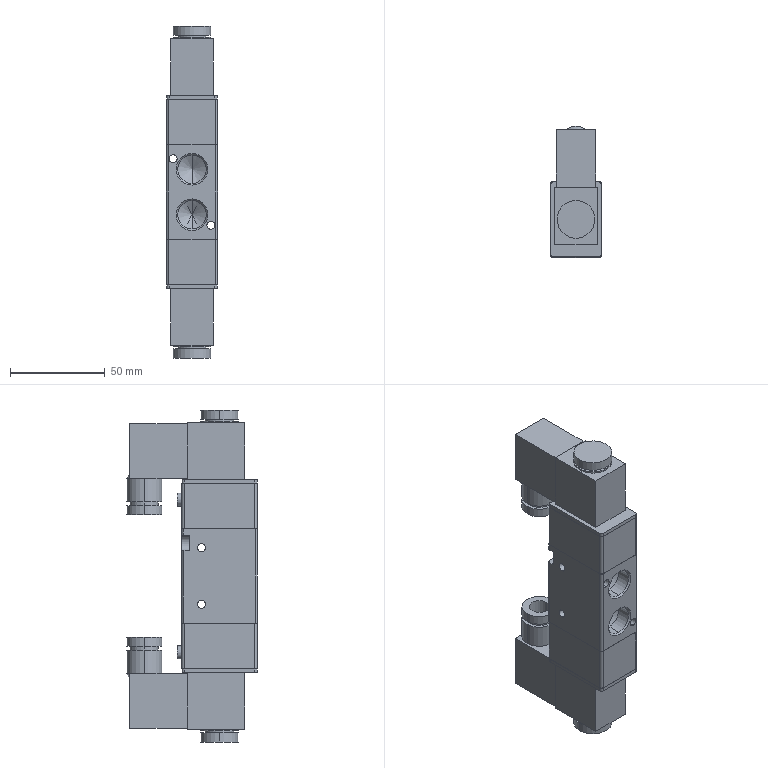Part | SolidWorks | features AEMSimFeature 1 | 1 solid | 152 faces | box 27 x 69.2 x 175.4 mm | volume 190277 mm3 | cylinder 70 | plane 68 | cone 14 | commonest cylinder face diameters 2.4 x22 4.3 x8 15 x8 18.6 x8 20 x8 14.95 x6